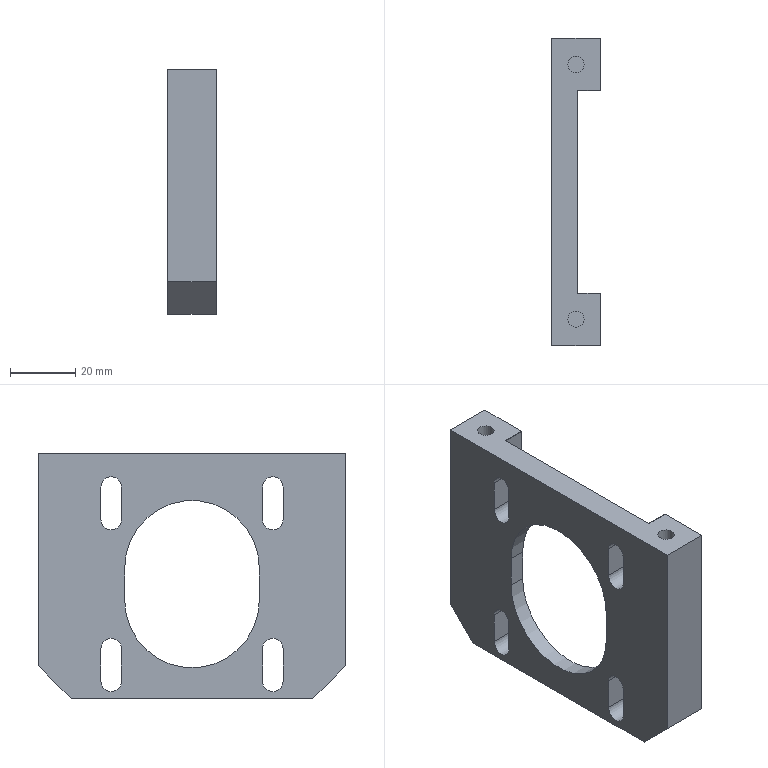Part | 1 solid | 45 faces | box 15 x 94 x 75 mm | volume 51821 mm3 | plane 31 | cylinder 14 | commonest cylinder face diameters 6.3 x8 5 x2 41.2 x2 50.6 x2
STEP:
#1=CARTESIAN_POINT('',(-74.806,502.943,-274.3));
#2=VERTEX_POINT('',#1);
#3=CARTESIAN_POINT('',(-77.306,502.943,-274.3));
#4=DIRECTION('',(0.,0.,1.));
#5=DIRECTION('',(1.,0.,0.));
#6=AXIS2_PLACEMENT_3D('',#3,#4,#5);
#7=CIRCLE('',#6,2.5);
#8=EDGE_CURVE('',#2,#2,#7,.T.);
#9=ORIENTED_EDGE('',*,*,#8,.T.);
#10=EDGE_LOOP('',(#9));
#11=FACE_BOUND('',#10,.T.);
#12=CARTESIAN_POINT('',(-74.806,502.943,-289.3));
#13=VERTEX_POINT('',#12);
#14=CARTESIAN_POINT('',(-77.306,502.943,-289.3));
#15=DIRECTION('',(0.,0.,-1.));
#16=DIRECTION('',(1.,0.,0.));
#17=AXIS2_PLACEMENT_3D('',#14,#15,#16);
#18=CIRCLE('',#17,2.5);
#19=EDGE_CURVE('',#13,#13,#18,.T.);
#20=ORIENTED_EDGE('',*,*,#19,.T.);
#21=EDGE_LOOP('',(#20));
#22=FACE_BOUND('',#21,.T.);
#23=CARTESIAN_POINT('',(-77.306,502.943,-274.3));
#24=DIRECTION('',(0.,0.,-1.));
#25=DIRECTION('',(1.,0.,0.));
#26=AXIS2_PLACEMENT_3D('',#23,#24,#25);
#27=CYLINDRICAL_SURFACE('',#26,2.5);
#28=ADVANCED_FACE('',(#11,#22),#27,.F.);
#29=ORIENTED_EDGE('',*,*,#19,.F.);
#30=EDGE_LOOP('',(#29));
#31=FACE_BOUND('',#30,.T.);
#32=CARTESIAN_POINT('',(-77.306,502.943,-289.3));
#33=DIRECTION('',(0.,0.,-1.));
#34=DIRECTION('',(-1.,0.,0.));
#35=AXIS2_PLACEMENT_3D('',#32,#33,#34);
#36=PLANE('',#35);
#37=ADVANCED_FACE('',(#31),#36,.F.);
#38=CARTESIAN_POINT('',(-74.806,424.943,-274.3));
#39=VERTEX_POINT('',#38);
#40=CARTESIAN_POINT('',(-77.306,424.943,-274.3));
#41=DIRECTION('',(0.,0.,1.));
#42=DIRECTION('',(1.,0.,0.));
#43=AXIS2_PLACEMENT_3D('',#40,#41,#42);
#44=CIRCLE('',#43,2.5);
#45=EDGE_CURVE('',#39,#39,#44,.T.);
#46=ORIENTED_EDGE('',*,*,#45,.T.);
#47=EDGE_LOOP('',(#46));
#48=FACE_BOUND('',#47,.T.);
#49=CARTESIAN_POINT('',(-79.806,424.943,-289.3));
#50=VERTEX_POINT('',#49);
#51=CARTESIAN_POINT('',(-77.306,424.943,-289.3));
#52=DIRECTION('',(0.,0.,-1.));
#53=DIRECTION('',(-1.,0.,0.));
#54=AXIS2_PLACEMENT_3D('',#51,#52,#53);
#55=CIRCLE('',#54,2.5);
#56=EDGE_CURVE('',#50,#50,#55,.T.);
#57=ORIENTED_EDGE('',*,*,#56,.T.);
#58=EDGE_LOOP('',(#57));
#59=FACE_BOUND('',#58,.T.);
#60=CARTESIAN_POINT('',(-77.306,424.943,-274.3));
#61=DIRECTION('',(0.,0.,-1.));
#62=DIRECTION('',(1.,0.,0.));
#63=AXIS2_PLACEMENT_3D('',#60,#61,#62);
#64=CYLINDRICAL_SURFACE('',#63,2.5);
#65=ADVANCED_FACE('',(#48,#59),#64,.F.);
#66=ORIENTED_EDGE('',*,*,#56,.F.);
#67=EDGE_LOOP('',(#66));
#68=FACE_BOUND('',#67,.T.);
#69=CARTESIAN_POINT('',(-77.306,502.943,-289.3));
#70=DIRECTION('',(0.,0.,-1.));
#71=DIRECTION('',(-1.,0.,0.));
#72=AXIS2_PLACEMENT_3D('',#69,#70,#71);
#73=PLANE('',#72);
#74=ADVANCED_FACE('',(#68),#73,.F.);
#75=CARTESIAN_POINT('',(-69.806,416.943,-339.3));
#76=VERTEX_POINT('',#75);
#77=CARTESIAN_POINT('',(-69.806,426.943,-349.3));
#78=VERTEX_POINT('',#77);
#79=CARTESIAN_POINT('',(-69.806,447.943,-370.3));
#80=DIRECTION('',(0.,0.7071,-0.7071));
#81=VECTOR('',#80,1000.);
#82=LINE('',#79,#81);
#83=EDGE_CURVE('',#76,#78,#82,.T.);
#84=ORIENTED_EDGE('',*,*,#83,.F.);
#85=CARTESIAN_POINT('',(-84.806,416.943,-339.3));
#86=VERTEX_POINT('',#85);
#87=CARTESIAN_POINT('',(-74.806,416.943,-339.3));
#88=DIRECTION('',(1.,0.,0.));
#89=VECTOR('',#88,1000.);
#90=LINE('',#87,#89);
#91=EDGE_CURVE('',#86,#76,#90,.T.);
#92=ORIENTED_EDGE('',*,*,#91,.F.);
#93=CARTESIAN_POINT('',(-84.806,426.943,-349.3));
#94=VERTEX_POINT('',#93);
#95=CARTESIAN_POINT('',(-84.806,447.943,-370.3));
#96=DIRECTION('',(0.,-0.7071,0.7071));
#97=VECTOR('',#96,1000.);
#98=LINE('',#95,#97);
#99=EDGE_CURVE('',#94,#86,#98,.T.);
#100=ORIENTED_EDGE('',*,*,#99,.F.);
#101=CARTESIAN_POINT('',(25.994,426.943,-349.3));
#102=DIRECTION('',(-1.,0.,0.));
#103=VECTOR('',#102,1000.);
#104=LINE('',#101,#103);
#105=EDGE_CURVE('',#78,#94,#104,.T.);
#106=ORIENTED_EDGE('',*,*,#105,.F.);
#107=EDGE_LOOP('',(#84,#92,#100,#106));
#108=FACE_BOUND('',#107,.T.);
#109=CARTESIAN_POINT('',(25.994,426.943,-349.3));
#110=DIRECTION('',(0.,0.7071,0.7071));
#111=DIRECTION('',(-1.,0.,0.));
#112=AXIS2_PLACEMENT_3D('',#109,#110,#111);
#113=PLANE('',#112);
#114=ADVANCED_FACE('',(#108),#113,.F.);
#115=CARTESIAN_POINT('',(-84.806,510.943,-339.3));
#116=VERTEX_POINT('',#115);
#117=CARTESIAN_POINT('',(-84.806,500.943,-349.3));
#118=VERTEX_POINT('',#117);
#119=CARTESIAN_POINT('',(-84.806,479.943,-370.3));
#120=DIRECTION('',(0.,-0.7071,-0.7071));
#121=VECTOR('',#120,1000.);
#122=LINE('',#119,#121);
#123=EDGE_CURVE('',#116,#118,#122,.T.);
#124=ORIENTED_EDGE('',*,*,#123,.F.);
#125=CARTESIAN_POINT('',(-69.806,510.943,-339.3));
#126=VERTEX_POINT('',#125);
#127=CARTESIAN_POINT('',(-74.806,510.943,-339.3));
#128=DIRECTION('',(-1.,0.,0.));
#129=VECTOR('',#128,1000.);
#130=LINE('',#127,#129);
#131=EDGE_CURVE('',#126,#116,#130,.T.);
#132=ORIENTED_EDGE('',*,*,#131,.F.);
#133=CARTESIAN_POINT('',(-69.806,500.943,-349.3));
#134=VERTEX_POINT('',#133);
#135=CARTESIAN_POINT('',(-69.806,479.943,-370.3));
#136=DIRECTION('',(0.,0.7071,0.7071));
#137=VECTOR('',#136,1000.);
#138=LINE('',#135,#137);
#139=EDGE_CURVE('',#134,#126,#138,.T.);
#140=ORIENTED_EDGE('',*,*,#139,.F.);
#141=CARTESIAN_POINT('',(25.994,500.943,-349.3));
#142=DIRECTION('',(1.,0.,0.));
#143=VECTOR('',#142,1000.);
#144=LINE('',#141,#143);
#145=EDGE_CURVE('',#118,#134,#144,.T.);
#146=ORIENTED_EDGE('',*,*,#145,.F.);
#147=EDGE_LOOP('',(#124,#132,#140,#146));
#148=FACE_BOUND('',#147,.T.);
#149=CARTESIAN_POINT('',(25.994,500.943,-349.3));
#150=DIRECTION('',(0.,-0.7071,0.7071));
#151=DIRECTION('',(1.,0.,0.));
#152=AXIS2_PLACEMENT_3D('',#149,#150,#151);
#153=PLANE('',#152);
#154=ADVANCED_FACE('',(#148),#153,.F.);
#155=CARTESIAN_POINT('',(-76.806,436.044,-344.049));
#156=VERTEX_POINT('',#155);
#157=CARTESIAN_POINT('',(-76.806,442.344,-344.049));
#158=VERTEX_POINT('',#157);
#159=CARTESIAN_POINT('',(-76.806,439.194,-344.049));
#160=DIRECTION('',(1.,0.,0.));
#161=DIRECTION('',(0.,1.,0.));
#162=AXIS2_PLACEMENT_3D('',#159,#160,#161);
#163=CIRCLE('',#162,3.15);
#164=EDGE_CURVE('',#156,#158,#163,.T.);
#165=ORIENTED_EDGE('',*,*,#164,.T.);
#166=CARTESIAN_POINT('',(-84.806,442.344,-344.049));
#167=VERTEX_POINT('',#166);
#168=CARTESIAN_POINT('',(-80.806,442.344,-344.049));
#169=DIRECTION('',(1.,0.,0.));
#170=VECTOR('',#169,1000.);
#171=LINE('',#168,#170);
#172=EDGE_CURVE('',#167,#158,#171,.T.);
#173=ORIENTED_EDGE('',*,*,#172,.F.);
#174=CARTESIAN_POINT('',(-84.806,436.044,-344.049));
#175=VERTEX_POINT('',#174);
#176=CARTESIAN_POINT('',(-84.806,439.194,-344.049));
#177=DIRECTION('',(-1.,0.,0.));
#178=DIRECTION('',(0.,-1.,0.));
#179=AXIS2_PLACEMENT_3D('',#176,#177,#178);
#180=CIRCLE('',#179,3.15);
#181=EDGE_CURVE('',#167,#175,#180,.T.);
#182=ORIENTED_EDGE('',*,*,#181,.T.);
#183=CARTESIAN_POINT('',(-80.806,436.044,-344.049));
#184=DIRECTION('',(-1.,0.,0.));
#185=VECTOR('',#184,1000.);
#186=LINE('',#183,#185);
#187=EDGE_CURVE('',#156,#175,#186,.T.);
#188=ORIENTED_EDGE('',*,*,#187,.F.);
#189=EDGE_LOOP('',(#165,#173,#182,#188));
#190=FACE_BOUND('',#189,.T.);
#191=CARTESIAN_POINT('',(-80.806,439.194,-344.049));
#192=DIRECTION('',(-1.,0.,0.));
#193=DIRECTION('',(0.,-1.,0.));
#194=AXIS2_PLACEMENT_3D('',#191,#192,#193);
#195=CYLINDRICAL_SURFACE('',#194,3.15);
#196=ADVANCED_FACE('',(#190),#195,.F.);
#197=CARTESIAN_POINT('',(-76.806,442.344,-334.049));
#198=VERTEX_POINT('',#197);
#199=CARTESIAN_POINT('',(-76.806,436.044,-334.049));
#200=VERTEX_POINT('',#199);
#201=CARTESIAN_POINT('',(-76.806,439.194,-334.049));
#202=DIRECTION('',(1.,0.,0.));
#203=DIRECTION('',(0.,1.,0.));
#204=AXIS2_PLACEMENT_3D('',#201,#202,#203);
#205=CIRCLE('',#204,3.15);
#206=EDGE_CURVE('',#198,#200,#205,.T.);
#207=ORIENTED_EDGE('',*,*,#206,.T.);
#208=CARTESIAN_POINT('',(-84.806,436.044,-334.049));
#209=VERTEX_POINT('',#208);
#210=CARTESIAN_POINT('',(-80.806,436.044,-334.049));
#211=DIRECTION('',(1.,0.,0.));
#212=VECTOR('',#211,1000.);
#213=LINE('',#210,#212);
#214=EDGE_CURVE('',#209,#200,#213,.T.);
#215=ORIENTED_EDGE('',*,*,#214,.F.);
#216=CARTESIAN_POINT('',(-84.806,442.344,-334.049));
#217=VERTEX_POINT('',#216);
#218=CARTESIAN_POINT('',(-84.806,439.194,-334.049));
#219=DIRECTION('',(-1.,0.,0.));
#220=DIRECTION('',(0.,-1.,0.));
#221=AXIS2_PLACEMENT_3D('',#218,#219,#220);
#222=CIRCLE('',#221,3.15);
#223=EDGE_CURVE('',#209,#217,#222,.T.);
#224=ORIENTED_EDGE('',*,*,#223,.T.);
#225=CARTESIAN_POINT('',(-80.806,442.344,-334.049));
#226=DIRECTION('',(-1.,0.,0.));
#227=VECTOR('',#226,1000.);
#228=LINE('',#225,#227);
#229=EDGE_CURVE('',#198,#217,#228,.T.);
#230=ORIENTED_EDGE('',*,*,#229,.F.);
#231=EDGE_LOOP('',(#207,#215,#224,#230));
#232=FACE_BOUND('',#231,.T.);
#233=CARTESIAN_POINT('',(-80.806,439.194,-334.049));
#234=DIRECTION('',(1.,0.,0.));
#235=DIRECTION('',(0.,1.,0.));
#236=AXIS2_PLACEMENT_3D('',#233,#234,#235);
#237=CYLINDRICAL_SURFACE('',#236,3.15);
#238=ADVANCED_FACE('',(#232),#237,.F.);
#239=CARTESIAN_POINT('',(-84.806,442.344,-339.049));
#240=DIRECTION('',(0.,0.,-1.));
#241=VECTOR('',#240,1000.);
#242=LINE('',#239,#241);
#243=EDGE_CURVE('',#217,#167,#242,.T.);
#244=ORIENTED_EDGE('',*,*,#243,.T.);
#245=ORIENTED_EDGE('',*,*,#172,.T.);
#246=CARTESIAN_POINT('',(-76.806,442.344,-354.3));
#247=DIRECTION('',(0.,0.,1.));
#248=VECTOR('',#247,1000.);
#249=LINE('',#246,#248);
#250=EDGE_CURVE('',#158,#198,#249,.T.);
#251=ORIENTED_EDGE('',*,*,#250,.T.);
#252=ORIENTED_EDGE('',*,*,#229,.T.);
#253=EDGE_LOOP('',(#244,#245,#251,#252));
#254=FACE_BOUND('',#253,.T.);
#255=CARTESIAN_POINT('',(-80.806,442.344,-339.049));
#256=DIRECTION('',(0.,1.,0.));
#257=DIRECTION('',(-1.,0.,0.));
#258=AXIS2_PLACEMENT_3D('',#255,#256,#257);
#259=PLANE('',#258);
#260=ADVANCED_FACE('',(#254),#259,.F.);
#261=CARTESIAN_POINT('',(-84.806,436.044,-339.049));
#262=DIRECTION('',(0.,0.,1.));
#263=VECTOR('',#262,1000.);
#264=LINE('',#261,#263);
#265=EDGE_CURVE('',#175,#209,#264,.T.);
#266=ORIENTED_EDGE('',*,*,#265,.T.);
#267=ORIENTED_EDGE('',*,*,#214,.T.);
#268=CARTESIAN_POINT('',(-76.806,436.044,-354.3));
#269=DIRECTION('',(0.,0.,-1.));
#270=VECTOR('',#269,1000.);
#271=LINE('',#268,#270);
#272=EDGE_CURVE('',#200,#156,#271,.T.);
#273=ORIENTED_EDGE('',*,*,#272,.T.);
#274=ORIENTED_EDGE('',*,*,#187,.T.);
#275=EDGE_LOOP('',(#266,#267,#273,#274));
#276=FACE_BOUND('',#275,.T.);
#277=CARTESIAN_POINT('',(-80.806,436.044,-339.049));
#278=DIRECTION('',(0.,-1.,0.));
#279=DIRECTION('',(1.,0.,0.));
#280=AXIS2_PLACEMENT_3D('',#277,#278,#279);
#281=PLANE('',#280);
#282=ADVANCED_FACE('',(#276),#281,.F.);
#283=CARTESIAN_POINT('',(-76.806,436.044,-294.551));
#284=VERTEX_POINT('',#283);
#285=CARTESIAN_POINT('',(-76.806,442.344,-294.551));
#286=VERTEX_POINT('',#285);
#287=CARTESIAN_POINT('',(-76.806,439.194,-294.551));
#288=DIRECTION('',(1.,0.,0.));
#289=DIRECTION('',(0.,1.,0.));
#290=AXIS2_PLACEMENT_3D('',#287,#288,#289);
#291=CIRCLE('',#290,3.15);
#292=EDGE_CURVE('',#284,#286,#291,.T.);
#293=ORIENTED_EDGE('',*,*,#292,.T.);
#294=CARTESIAN_POINT('',(-84.806,442.344,-294.551));
#295=VERTEX_POINT('',#294);
#296=CARTESIAN_POINT('',(-80.806,442.344,-294.551));
#297=DIRECTION('',(1.,0.,0.));
#298=VECTOR('',#297,1000.);
#299=LINE('',#296,#298);
#300=EDGE_CURVE('',#295,#286,#299,.T.);
#301=ORIENTED_EDGE('',*,*,#300,.F.);
#302=CARTESIAN_POINT('',(-84.806,436.044,-294.551));
#303=VERTEX_POINT('',#302);
#304=CARTESIAN_POINT('',(-84.806,439.194,-294.551));
#305=DIRECTION('',(-1.,0.,0.));
#306=DIRECTION('',(0.,-1.,0.));
#307=AXIS2_PLACEMENT_3D('',#304,#305,#306);
#308=CIRCLE('',#307,3.15);
#309=EDGE_CURVE('',#295,#303,#308,.T.);
#310=ORIENTED_EDGE('',*,*,#309,.T.);
#311=CARTESIAN_POINT('',(-80.806,436.044,-294.551));
#312=DIRECTION('',(-1.,0.,0.));
#313=VECTOR('',#312,1000.);
#314=LINE('',#311,#313);
#315=EDGE_CURVE('',#284,#303,#314,.T.);
#316=ORIENTED_EDGE('',*,*,#315,.F.);
#317=EDGE_LOOP('',(#293,#301,#310,#316));
#318=FACE_BOUND('',#317,.T.);
#319=CARTESIAN_POINT('',(-80.806,439.194,-294.551));
#320=DIRECTION('',(-1.,0.,0.));
#321=DIRECTION('',(0.,-1.,0.));
#322=AXIS2_PLACEMENT_3D('',#319,#320,#321);
#323=CYLINDRICAL_SURFACE('',#322,3.15);
#324=ADVANCED_FACE('',(#318),#323,.F.);
#325=CARTESIAN_POINT('',(-76.806,442.344,-284.551));
#326=VERTEX_POINT('',#325);
#327=CARTESIAN_POINT('',(-76.806,436.044,-284.551));
#328=VERTEX_POINT('',#327);
#329=CARTESIAN_POINT('',(-76.806,439.194,-284.551));
#330=DIRECTION('',(1.,0.,0.));
#331=DIRECTION('',(0.,1.,0.));
#332=AXIS2_PLACEMENT_3D('',#329,#330,#331);
#333=CIRCLE('',#332,3.15);
#334=EDGE_CURVE('',#326,#328,#333,.T.);
#335=ORIENTED_EDGE('',*,*,#334,.T.);
#336=CARTESIAN_POINT('',(-84.806,436.044,-284.551));
#337=VERTEX_POINT('',#336);
#338=CARTESIAN_POINT('',(-80.806,436.044,-284.551));
#339=DIRECTION('',(1.,0.,0.));
#340=VECTOR('',#339,1000.);
#341=LINE('',#338,#340);
#342=EDGE_CURVE('',#337,#328,#341,.T.);
#343=ORIENTED_EDGE('',*,*,#342,.F.);
#344=CARTESIAN_POINT('',(-84.806,442.344,-284.551));
#345=VERTEX_POINT('',#344);
#346=CARTESIAN_POINT('',(-84.806,439.194,-284.551));
#347=DIRECTION('',(-1.,0.,0.));
#348=DIRECTION('',(0.,-1.,0.));
#349=AXIS2_PLACEMENT_3D('',#346,#347,#348);
#350=CIRCLE('',#349,3.15);
#351=EDGE_CURVE('',#337,#345,#350,.T.);
#352=ORIENTED_EDGE('',*,*,#351,.T.);
#353=CARTESIAN_POINT('',(-80.806,442.344,-284.551));
#354=DIRECTION('',(-1.,0.,0.));
#355=VECTOR('',#354,1000.);
#356=LINE('',#353,#355);
#357=EDGE_CURVE('',#326,#345,#356,.T.);
#358=ORIENTED_EDGE('',*,*,#357,.F.);
#359=EDGE_LOOP('',(#335,#343,#352,#358));
#360=FACE_BOUND('',#359,.T.);
#361=CARTESIAN_POINT('',(-80.806,439.194,-284.551));
#362=DIRECTION('',(1.,0.,0.));
#363=DIRECTION('',(0.,1.,0.));
#364=AXIS2_PLACEMENT_3D('',#361,#362,#363);
#365=CYLINDRICAL_SURFACE('',#364,3.15);
#366=ADVANCED_FACE('',(#360),#365,.F.);
#367=CARTESIAN_POINT('',(-84.806,442.344,-339.049));
#368=DIRECTION('',(0.,0.,-1.));
#369=VECTOR('',#368,1000.);
#370=LINE('',#367,#369);
#371=EDGE_CURVE('',#345,#295,#370,.T.);
#372=ORIENTED_EDGE('',*,*,#371,.T.);
#373=ORIENTED_EDGE('',*,*,#300,.T.);
#374=CARTESIAN_POINT('',(-76.806,442.344,-339.049));
#375=DIRECTION('',(0.,0.,1.));
#376=VECTOR('',#375,1000.);
#377=LINE('',#374,#376);
#378=EDGE_CURVE('',#286,#326,#377,.T.);
#379=ORIENTED_EDGE('',*,*,#378,.T.);
#380=ORIENTED_EDGE('',*,*,#357,.T.);
#381=EDGE_LOOP('',(#372,#373,#379,#380));
#382=FACE_BOUND('',#381,.T.);
#383=CARTESIAN_POINT('',(-80.806,442.344,-339.049));
#384=DIRECTION('',(0.,1.,0.));
#385=DIRECTION('',(-1.,0.,0.));
#386=AXIS2_PLACEMENT_3D('',#383,#384,#385);
#387=PLANE('',#386);
#388=ADVANCED_FACE('',(#382),#387,.F.);
#389=CARTESIAN_POINT('',(-84.806,436.044,-339.049));
#390=DIRECTION('',(0.,0.,1.));
#391=VECTOR('',#390,1000.);
#392=LINE('',#389,#391);
#393=EDGE_CURVE('',#303,#337,#392,.T.);
#394=ORIENTED_EDGE('',*,*,#393,.T.);
#395=ORIENTED_EDGE('',*,*,#342,.T.);
#396=CARTESIAN_POINT('',(-76.806,436.044,-339.049));
#397=DIRECTION('',(0.,0.,-1.));
#398=VECTOR('',#397,1000.);
#399=LINE('',#396,#398);
#400=EDGE_CURVE('',#328,#284,#399,.T.);
#401=ORIENTED_EDGE('',*,*,#400,.T.);
#402=ORIENTED_EDGE('',*,*,#315,.T.);
#403=EDGE_LOOP('',(#394,#395,#401,#402));
#404=FACE_BOUND('',#403,.T.);
#405=CARTESIAN_POINT('',(-80.806,436.044,-339.049));
#406=DIRECTION('',(0.,-1.,0.));
#407=DIRECTION('',(1.,0.,0.));
#408=AXIS2_PLACEMENT_3D('',#405,#406,#407);
#409=PLANE('',#408);
#410=ADVANCED_FACE('',(#404),#409,.F.);
#411=CARTESIAN_POINT('',(-76.806,485.542,-344.049));
#412=VERTEX_POINT('',#411);
#413=CARTESIAN_POINT('',(-76.806,491.842,-344.049));
#414=VERTEX_POINT('',#413);
#415=CARTESIAN_POINT('',(-76.806,488.692,-344.049));
#416=DIRECTION('',(1.,0.,0.));
#417=DIRECTION('',(0.,1.,0.));
#418=AXIS2_PLACEMENT_3D('',#415,#416,#417);
#419=CIRCLE('',#418,3.15);
#420=EDGE_CURVE('',#412,#414,#419,.T.);
#421=ORIENTED_EDGE('',*,*,#420,.T.);
#422=CARTESIAN_POINT('',(-84.806,491.842,-344.049));
#423=VERTEX_POINT('',#422);
#424=CARTESIAN_POINT('',(-80.806,491.842,-344.049));
#425=DIRECTION('',(1.,0.,0.));
#426=VECTOR('',#425,1000.);
#427=LINE('',#424,#426);
#428=EDGE_CURVE('',#423,#414,#427,.T.);
#429=ORIENTED_EDGE('',*,*,#428,.F.);
#430=CARTESIAN_POINT('',(-84.806,485.542,-344.049));
#431=VERTEX_POINT('',#430);
#432=CARTESIAN_POINT('',(-84.806,488.692,-344.049));
#433=DIRECTION('',(-1.,0.,0.));
#434=DIRECTION('',(0.,-1.,0.));
#435=AXIS2_PLACEMENT_3D('',#432,#433,#434);
#436=CIRCLE('',#435,3.15);
#437=EDGE_CURVE('',#423,#431,#436,.T.);
#438=ORIENTED_EDGE('',*,*,#437,.T.);
#439=CARTESIAN_POINT('',(-80.806,485.542,-344.049));
#440=DIRECTION('',(-1.,0.,0.));
#441=VECTOR('',#440,1000.);
#442=LINE('',#439,#441);
#443=EDGE_CURVE('',#412,#431,#442,.T.);
#444=ORIENTED_EDGE('',*,*,#443,.F.);
#445=EDGE_LOOP('',(#421,#429,#438,#444));
#446=FACE_BOUND('',#445,.T.);
#447=CARTESIAN_POINT('',(-80.806,488.692,-344.049));
#448=DIRECTION('',(-1.,0.,0.));
#449=DIRECTION('',(0.,-1.,0.));
#450=AXIS2_PLACEMENT_3D('',#447,#448,#449);
#451=CYLINDRICAL_SURFACE('',#450,3.15);
#452=ADVANCED_FACE('',(#446),#451,.F.);
#453=CARTESIAN_POINT('',(-76.806,491.842,-334.049));
#454=VERTEX_POINT('',#453);
#455=CARTESIAN_POINT('',(-76.806,485.542,-334.049));
#456=VERTEX_POINT('',#455);
#457=CARTESIAN_POINT('',(-76.806,488.692,-334.049));
#458=DIRECTION('',(1.,0.,0.));
#459=DIRECTION('',(0.,1.,0.));
#460=AXIS2_PLACEMENT_3D('',#457,#458,#459);
#461=CIRCLE('',#460,3.15);
#462=EDGE_CURVE('',#454,#456,#461,.T.);
#463=ORIENTED_EDGE('',*,*,#462,.T.);
#464=CARTESIAN_POINT('',(-84.806,485.542,-334.049));
#465=VERTEX_POINT('',#464);
#466=CARTESIAN_POINT('',(-80.806,485.542,-334.049));
#467=DIRECTION('',(1.,0.,0.));
#468=VECTOR('',#467,1000.);
#469=LINE('',#466,#468);
#470=EDGE_CURVE('',#465,#456,#469,.T.);
#471=ORIENTED_EDGE('',*,*,#470,.F.);
#472=CARTESIAN_POINT('',(-84.806,491.842,-334.049));
#473=VERTEX_POINT('',#472);
#474=CARTESIAN_POINT('',(-84.806,488.692,-334.049));
#475=DIRECTION('',(-1.,0.,0.));
#476=DIRECTION('',(0.,-1.,0.));
#477=AXIS2_PLACEMENT_3D('',#474,#475,#476);
#478=CIRCLE('',#477,3.15);
#479=EDGE_CURVE('',#465,#473,#478,.T.);
#480=ORIENTED_EDGE('',*,*,#479,.T.);
#481=CARTESIAN_POINT('',(-80.806,491.842,-334.049));
#482=DIRECTION('',(-1.,0.,0.));
#483=VECTOR('',#482,1000.);
#484=LINE('',#481,#483);
#485=EDGE_CURVE('',#454,#473,#484,.T.);
#486=ORIENTED_EDGE('',*,*,#485,.F.);
#487=EDGE_LOOP('',(#463,#471,#480,#486));
#488=FACE_BOUND('',#487,.T.);
#489=CARTESIAN_POINT('',(-80.806,488.692,-334.049));
#490=DIRECTION('',(1.,0.,0.));
#491=DIRECTION('',(0.,1.,0.));
#492=AXIS2_PLACEMENT_3D('',#489,#490,#491);
#493=CYLINDRICAL_SURFACE('',#492,3.15);
#494=ADVANCED_FACE('',(#488),#493,.F.);
#495=CARTESIAN_POINT('',(-84.806,491.842,-339.049));
#496=DIRECTION('',(0.,0.,-1.));
#497=VECTOR('',#496,1000.);
#498=LINE('',#495,#497);
#499=EDGE_CURVE('',#473,#423,#498,.T.);
#500=ORIENTED_EDGE('',*,*,#499,.T.);
#501=ORIENTED_EDGE('',*,*,#428,.T.);
#502=CARTESIAN_POINT('',(-76.806,491.842,-354.3));
#503=DIRECTION('',(0.,0.,1.));
#504=VECTOR('',#503,1000.);
#505=LINE('',#502,#504);
#506=EDGE_CURVE('',#414,#454,#505,.T.);
#507=ORIENTED_EDGE('',*,*,#506,.T.);
#508=ORIENTED_EDGE('',*,*,#485,.T.);
#509=EDGE_LOOP('',(#500,#501,#507,#508));
#510=FACE_BOUND('',#509,.T.);
#511=CARTESIAN_POINT('',(-80.806,491.842,-339.049));
#512=DIRECTION('',(0.,1.,0.));
#513=DIRECTION('',(-1.,0.,0.));
#514=AXIS2_PLACEMENT_3D('',#511,#512,#513);
#515=PLANE('',#514);
#516=ADVANCED_FACE('',(#510),#515,.F.);
#517=CARTESIAN_POINT('',(-84.806,485.542,-339.049));
#518=DIRECTION('',(0.,0.,1.));
#519=VECTOR('',#518,1000.);
#520=LINE('',#517,#519);
#521=EDGE_CURVE('',#431,#465,#520,.T.);
#522=ORIENTED_EDGE('',*,*,#521,.T.);
#523=ORIENTED_EDGE('',*,*,#470,.T.);
#524=CARTESIAN_POINT('',(-76.806,485.542,-354.3));
#525=DIRECTION('',(0.,0.,-1.));
#526=VECTOR('',#525,1000.);
#527=LINE('',#524,#526);
#528=EDGE_CURVE('',#456,#412,#527,.T.);
#529=ORIENTED_EDGE('',*,*,#528,.T.);
#530=ORIENTED_EDGE('',*,*,#443,.T.);
#531=EDGE_LOOP('',(#522,#523,#529,#530));
#532=FACE_BOUND('',#531,.T.);
#533=CARTESIAN_POINT('',(-80.806,485.542,-339.049));
#534=DIRECTION('',(0.,-1.,0.));
#535=DIRECTION('',(1.,0.,0.));
#536=AXIS2_PLACEMENT_3D('',#533,#534,#535);
#537=PLANE('',#536);
#538=ADVANCED_FACE('',(#532),#537,.F.);
#539=CARTESIAN_POINT('',(-76.806,485.542,-294.551));
#540=VERTEX_POINT('',#539);
#541=CARTESIAN_POINT('',(-76.806,491.842,-294.551));
#542=VERTEX_POINT('',#541);
#543=CARTESIAN_POINT('',(-76.806,488.692,-294.551));
#544=DIRECTION('',(1.,0.,0.));
#545=DIRECTION('',(0.,1.,0.));
#546=AXIS2_PLACEMENT_3D('',#543,#544,#545);
#547=CIRCLE('',#546,3.15);
#548=EDGE_CURVE('',#540,#542,#547,.T.);
#549=ORIENTED_EDGE('',*,*,#548,.T.);
#550=CARTESIAN_POINT('',(-84.806,491.842,-294.551));
#551=VERTEX_POINT('',#550);
#552=CARTESIAN_POINT('',(-80.806,491.842,-294.551));
#553=DIRECTION('',(1.,0.,0.));
#554=VECTOR('',#553,1000.);
#555=LINE('',#552,#554);
#556=EDGE_CURVE('',#551,#542,#555,.T.);
#557=ORIENTED_EDGE('',*,*,#556,.F.);
#558=CARTESIAN_POINT('',(-84.806,485.542,-294.551));
#559=VERTEX_POINT('',#558);
#560=CARTESIAN_POINT('',(-84.806,488.692,-294.551));
#561=DIRECTION('',(-1.,0.,0.));
#562=DIRECTION('',(0.,-1.,0.));
#563=AXIS2_PLACEMENT_3D('',#560,#561,#562);
#564=CIRCLE('',#563,3.15);
#565=EDGE_CURVE('',#551,#559,#564,.T.);
#566=ORIENTED_EDGE('',*,*,#565,.T.);
#567=CARTESIAN_POINT('',(-80.806,485.542,-294.551));
#568=DIRECTION('',(-1.,0.,0.));
#569=VECTOR('',#568,1000.);
#570=LINE('',#567,#569);
#571=EDGE_CURVE('',#540,#559,#570,.T.);
#572=ORIENTED_EDGE('',*,*,#571,.F.);
#573=EDGE_LOOP('',(#549,#557,#566,#572));
#574=FACE_BOUND('',#573,.T.);
#575=CARTESIAN_POINT('',(-80.806,488.692,-294.551));
#576=DIRECTION('',(-1.,0.,0.));
#577=DIRECTION('',(0.,-1.,0.));
#578=AXIS2_PLACEMENT_3D('',#575,#576,#577);
#579=CYLINDRICAL_SURFACE('',#578,3.15);
#580=ADVANCED_FACE('',(#574),#579,.F.);
#581=CARTESIAN_POINT('',(-76.806,491.842,-284.551));
#582=VERTEX_POINT('',#581);
#583=CARTESIAN_POINT('',(-76.806,485.542,-284.551));
#584=VERTEX_POINT('',#583);
#585=CARTESIAN_POINT('',(-76.806,488.692,-284.551));
#586=DIRECTION('',(1.,0.,0.));
#587=DIRECTION('',(0.,1.,0.));
#588=AXIS2_PLACEMENT_3D('',#585,#586,#587);
#589=CIRCLE('',#588,3.15);
#590=EDGE_CURVE('',#582,#584,#589,.T.);
#591=ORIENTED_EDGE('',*,*,#590,.T.);
#592=CARTESIAN_POINT('',(-84.806,485.542,-284.551));
#593=VERTEX_POINT('',#592);
#594=CARTESIAN_POINT('',(-80.806,485.542,-284.551));
#595=DIRECTION('',(1.,0.,0.));
#596=VECTOR('',#595,1000.);
#597=LINE('',#594,#596);
#598=EDGE_CURVE('',#593,#584,#597,.T.);
#599=ORIENTED_EDGE('',*,*,#598,.F.);
#600=CARTESIAN_POINT('',(-84.806,491.842,-284.551));
#601=VERTEX_POINT('',#600);
#602=CARTESIAN_POINT('',(-84.806,488.692,-284.551));
#603=DIRECTION('',(-1.,0.,0.));
#604=DIRECTION('',(0.,-1.,0.));
#605=AXIS2_PLACEMENT_3D('',#602,#603,#604);
#606=CIRCLE('',#605,3.15);
#607=EDGE_CURVE('',#593,#601,#606,.T.);
#608=ORIENTED_EDGE('',*,*,#607,.T.);
#609=CARTESIAN_POINT('',(-80.806,491.842,-284.551));
#610=DIRECTION('',(-1.,0.,0.));
#611=VECTOR('',#610,1000.);
#612=LINE('',#609,#611);
#613=EDGE_CURVE('',#582,#601,#612,.T.);
#614=ORIENTED_EDGE('',*,*,#613,.F.);
#615=EDGE_LOOP('',(#591,#599,#608,#614));
#616=FACE_BOUND('',#615,.T.);
#617=CARTESIAN_POINT('',(-80.806,488.692,-284.551));
#618=DIRECTION('',(1.,0.,0.));
#619=DIRECTION('',(0.,1.,0.));
#620=AXIS2_PLACEMENT_3D('',#617,#618,#619);
#621=CYLINDRICAL_SURFACE('',#620,3.15);
#622=ADVANCED_FACE('',(#616),#621,.F.);
#623=CARTESIAN_POINT('',(-84.806,491.842,-339.049));
#624=DIRECTION('',(0.,0.,-1.));
#625=VECTOR('',#624,1000.);
#626=LINE('',#623,#625);
#627=EDGE_CURVE('',#601,#551,#626,.T.);
#628=ORIENTED_EDGE('',*,*,#627,.T.);
#629=ORIENTED_EDGE('',*,*,#556,.T.);
#630=CARTESIAN_POINT('',(-76.806,491.842,-339.049));
#631=DIRECTION('',(0.,0.,1.));
#632=VECTOR('',#631,1000.);
#633=LINE('',#630,#632);
#634=EDGE_CURVE('',#542,#582,#633,.T.);
#635=ORIENTED_EDGE('',*,*,#634,.T.);
#636=ORIENTED_EDGE('',*,*,#613,.T.);
#637=EDGE_LOOP('',(#628,#629,#635,#636));
#638=FACE_BOUND('',#637,.T.);
#639=CARTESIAN_POINT('',(-80.806,491.842,-339.049));
#640=DIRECTION('',(0.,1.,0.));
#641=DIRECTION('',(-1.,0.,0.));
#642=AXIS2_PLACEMENT_3D('',#639,#640,#641);
#643=PLANE('',#642);
#644=ADVANCED_FACE('',(#638),#643,.F.);
#645=CARTESIAN_POINT('',(-84.806,485.542,-339.049));
#646=DIRECTION('',(0.,0.,1.));
#647=VECTOR('',#646,1000.);
#648=LINE('',#645,#647);
#649=EDGE_CURVE('',#559,#593,#648,.T.);
#650=ORIENTED_EDGE('',*,*,#649,.T.);
#651=ORIENTED_EDGE('',*,*,#598,.T.);
#652=CARTESIAN_POINT('',(-76.806,485.542,-339.049));
#653=DIRECTION('',(0.,0.,-1.));
#654=VECTOR('',#653,1000.);
#655=LINE('',#652,#654);
#656=EDGE_CURVE('',#584,#540,#655,.T.);
#657=ORIENTED_EDGE('',*,*,#656,.T.);
#658=ORIENTED_EDGE('',*,*,#571,.T.);
#659=EDGE_LOOP('',(#650,#651,#657,#658));
#660=FACE_BOUND('',#659,.T.);
#661=CARTESIAN_POINT('',(-80.806,485.542,-339.049));
#662=DIRECTION('',(0.,-1.,0.));
#663=DIRECTION('',(1.,0.,0.));
#664=AXIS2_PLACEMENT_3D('',#661,#662,#663);
#665=PLANE('',#664);
#666=ADVANCED_FACE('',(#660),#665,.F.);
#667=CARTESIAN_POINT('',(-84.806,443.343,-309.3));
#668=VERTEX_POINT('',#667);
#669=CARTESIAN_POINT('',(-79.806,443.343,-309.3));
#670=VERTEX_POINT('',#669);
#671=CARTESIAN_POINT('',(-82.306,443.343,-309.3));
#672=DIRECTION('',(1.,0.,0.));
#673=VECTOR('',#672,1000.);
#674=LINE('',#671,#673);
#675=EDGE_CURVE('',#668,#670,#674,.T.);
#676=ORIENTED_EDGE('',*,*,#675,.F.);
#677=CARTESIAN_POINT('',(-84.806,484.543,-309.3));
#678=VERTEX_POINT('',#677);
#679=CARTESIAN_POINT('',(-84.806,463.943,-309.3));
#680=DIRECTION('',(-1.,0.,0.));
#681=DIRECTION('',(0.,-1.,0.));
#682=AXIS2_PLACEMENT_3D('',#679,#680,#681);
#683=CIRCLE('',#682,20.6);
#684=EDGE_CURVE('',#668,#678,#683,.T.);
#685=ORIENTED_EDGE('',*,*,#684,.T.);
#686=CARTESIAN_POINT('',(-79.806,484.543,-309.3));
#687=VERTEX_POINT('',#686);
#688=CARTESIAN_POINT('',(-82.306,484.543,-309.3));
#689=DIRECTION('',(-1.,0.,0.));
#690=VECTOR('',#689,1000.);
#691=LINE('',#688,#690);
#692=EDGE_CURVE('',#687,#678,#691,.T.);
#693=ORIENTED_EDGE('',*,*,#692,.F.);
#694=CARTESIAN_POINT('',(-79.806,463.943,-309.3));
#695=DIRECTION('',(1.,0.,0.));
#696=DIRECTION('',(0.,1.,0.));
#697=AXIS2_PLACEMENT_3D('',#694,#695,#696);
#698=CIRCLE('',#697,20.6);
#699=EDGE_CURVE('',#687,#670,#698,.T.);
#700=ORIENTED_EDGE('',*,*,#699,.T.);
#701=EDGE_LOOP('',(#676,#685,#693,#700));
#702=FACE_BOUND('',#701,.T.);
#703=CARTESIAN_POINT('',(-82.306,463.943,-309.3));
#704=DIRECTION('',(1.,0.,0.));
#705=DIRECTION('',(0.,1.,0.));
#706=AXIS2_PLACEMENT_3D('',#703,#704,#705);
#707=CYLINDRICAL_SURFACE('',#706,20.6);
#708=ADVANCED_FACE('',(#702),#707,.F.);
#709=CARTESIAN_POINT('',(-84.806,484.543,-319.3));
#710=VERTEX_POINT('',#709);
#711=CARTESIAN_POINT('',(-79.806,484.543,-319.3));
#712=VERTEX_POINT('',#711);
#713=CARTESIAN_POINT('',(-82.306,484.543,-319.3));
#714=DIRECTION('',(1.,0.,0.));
#715=VECTOR('',#714,1000.);
#716=LINE('',#713,#715);
#717=EDGE_CURVE('',#710,#712,#716,.T.);
#718=ORIENTED_EDGE('',*,*,#717,.F.);
#719=CARTESIAN_POINT('',(-84.806,443.343,-319.3));
#720=VERTEX_POINT('',#719);
#721=CARTESIAN_POINT('',(-84.806,463.943,-319.3));
#722=DIRECTION('',(-1.,0.,0.));
#723=DIRECTION('',(0.,-1.,0.));
#724=AXIS2_PLACEMENT_3D('',#721,#722,#723);
#725=CIRCLE('',#724,20.6);
#726=EDGE_CURVE('',#710,#720,#725,.T.);
#727=ORIENTED_EDGE('',*,*,#726,.T.);
#728=CARTESIAN_POINT('',(-79.806,443.343,-319.3));
#729=VERTEX_POINT('',#728);
#730=CARTESIAN_POINT('',(-82.306,443.343,-319.3));
#731=DIRECTION('',(-1.,0.,0.));
#732=VECTOR('',#731,1000.);
#733=LINE('',#730,#732);
#734=EDGE_CURVE('',#729,#720,#733,.T.);
#735=ORIENTED_EDGE('',*,*,#734,.F.);
#736=CARTESIAN_POINT('',(-79.806,463.943,-319.3));
#737=DIRECTION('',(1.,0.,0.));
#738=DIRECTION('',(0.,1.,0.));
#739=AXIS2_PLACEMENT_3D('',#736,#737,#738);
#740=CIRCLE('',#739,20.6);
#741=EDGE_CURVE('',#729,#712,#740,.T.);
#742=ORIENTED_EDGE('',*,*,#741,.T.);
#743=EDGE_LOOP('',(#718,#727,#735,#742));
#744=FACE_BOUND('',#743,.T.);
#745=CARTESIAN_POINT('',(-82.306,463.943,-319.3));
#746=DIRECTION('',(1.,0.,0.));
#747=DIRECTION('',(0.,1.,0.));
#748=AXIS2_PLACEMENT_3D('',#745,#746,#747);
#749=CYLINDRICAL_SURFACE('',#748,20.6);
#750=ADVANCED_FACE('',(#744),#749,.F.);
#751=CARTESIAN_POINT('',(-84.806,484.543,-314.3));
#752=DIRECTION('',(0.,0.,-1.));
#753=VECTOR('',#752,1000.);
#754=LINE('',#751,#753);
#755=EDGE_CURVE('',#678,#710,#754,.T.);
#756=ORIENTED_EDGE('',*,*,#755,.T.);
#757=ORIENTED_EDGE('',*,*,#717,.T.);
#758=CARTESIAN_POINT('',(-79.806,484.543,-314.3));
#759=DIRECTION('',(0.,0.,1.));
#760=VECTOR('',#759,1000.);
#761=LINE('',#758,#760);
#762=EDGE_CURVE('',#712,#687,#761,.T.);
#763=ORIENTED_EDGE('',*,*,#762,.T.);
#764=ORIENTED_EDGE('',*,*,#692,.T.);
#765=EDGE_LOOP('',(#756,#757,#763,#764));
#766=FACE_BOUND('',#765,.T.);
#767=CARTESIAN_POINT('',(-82.306,484.543,-314.3));
#768=DIRECTION('',(0.,1.,0.));
#769=DIRECTION('',(-1.,0.,0.));
#770=AXIS2_PLACEMENT_3D('',#767,#768,#769);
#771=PLANE('',#770);
#772=ADVANCED_FACE('',(#766),#771,.F.);
#773=CARTESIAN_POINT('',(-84.806,443.343,-314.3));
#774=DIRECTION('',(0.,0.,1.));
#775=VECTOR('',#774,1000.);
#776=LINE('',#773,#775);
#777=EDGE_CURVE('',#720,#668,#776,.T.);
#778=ORIENTED_EDGE('',*,*,#777,.T.);
#779=ORIENTED_EDGE('',*,*,#675,.T.);
#780=CARTESIAN_POINT('',(-79.806,443.343,-314.3));
#781=DIRECTION('',(0.,0.,-1.));
#782=VECTOR('',#781,1000.);
#783=LINE('',#780,#782);
#784=EDGE_CURVE('',#670,#729,#783,.T.);
#785=ORIENTED_EDGE('',*,*,#784,.T.);
#786=ORIENTED_EDGE('',*,*,#734,.T.);
#787=EDGE_LOOP('',(#778,#779,#785,#786));
#788=FACE_BOUND('',#787,.T.);
#789=CARTESIAN_POINT('',(-82.306,443.343,-314.3));
#790=DIRECTION('',(0.,-1.,0.));
#791=DIRECTION('',(1.,0.,0.));
#792=AXIS2_PLACEMENT_3D('',#789,#790,#791);
#793=PLANE('',#792);
#794=ADVANCED_FACE('',(#788),#793,.F.);
#795=CARTESIAN_POINT('',(-76.806,438.643,-319.3));
#796=VERTEX_POINT('',#795);
#797=CARTESIAN_POINT('',(-79.806,438.643,-319.3));
#798=VERTEX_POINT('',#797);
#799=CARTESIAN_POINT('',(-78.306,438.643,-319.3));
#800=DIRECTION('',(-1.,0.,0.));
#801=VECTOR('',#800,1000.);
#802=LINE('',#799,#801);
#803=EDGE_CURVE('',#796,#798,#802,.T.);
#804=ORIENTED_EDGE('',*,*,#803,.F.);
#805=CARTESIAN_POINT('',(-76.806,489.243,-319.3));
#806=VERTEX_POINT('',#805);
#807=CARTESIAN_POINT('',(-76.806,463.943,-319.3));
#808=DIRECTION('',(1.,0.,0.));
#809=DIRECTION('',(0.,1.,0.));
#810=AXIS2_PLACEMENT_3D('',#807,#808,#809);
#811=CIRCLE('',#810,25.3);
#812=EDGE_CURVE('',#796,#806,#811,.T.);
#813=ORIENTED_EDGE('',*,*,#812,.T.);
#814=CARTESIAN_POINT('',(-79.806,489.243,-319.3));
#815=VERTEX_POINT('',#814);
#816=CARTESIAN_POINT('',(-78.306,489.243,-319.3));
#817=DIRECTION('',(1.,0.,0.));
#818=VECTOR('',#817,1000.);
#819=LINE('',#816,#818);
#820=EDGE_CURVE('',#815,#806,#819,.T.);
#821=ORIENTED_EDGE('',*,*,#820,.F.);
#822=CARTESIAN_POINT('',(-79.806,463.943,-319.3));
#823=DIRECTION('',(-1.,0.,0.));
#824=DIRECTION('',(0.,-1.,0.));
#825=AXIS2_PLACEMENT_3D('',#822,#823,#824);
#826=CIRCLE('',#825,25.3);
#827=EDGE_CURVE('',#815,#798,#826,.T.);
#828=ORIENTED_EDGE('',*,*,#827,.T.);
#829=EDGE_LOOP('',(#804,#813,#821,#828));
#830=FACE_BOUND('',#829,.T.);
#831=CARTESIAN_POINT('',(-78.306,463.943,-319.3));
#832=DIRECTION('',(-1.,0.,0.));
#833=DIRECTION('',(0.,-1.,0.));
#834=AXIS2_PLACEMENT_3D('',#831,#832,#833);
#835=CYLINDRICAL_SURFACE('',#834,25.3);
#836=ADVANCED_FACE('',(#830),#835,.F.);
#837=CARTESIAN_POINT('',(-79.806,438.643,-309.3));
#838=VERTEX_POINT('',#837);
#839=CARTESIAN_POINT('',(-76.806,438.643,-309.3));
#840=VERTEX_POINT('',#839);
#841=CARTESIAN_POINT('',(-78.306,438.643,-309.3));
#842=DIRECTION('',(1.,0.,0.));
#843=VECTOR('',#842,1000.);
#844=LINE('',#841,#843);
#845=EDGE_CURVE('',#838,#840,#844,.T.);
#846=ORIENTED_EDGE('',*,*,#845,.F.);
#847=CARTESIAN_POINT('',(-79.806,489.243,-309.3));
#848=VERTEX_POINT('',#847);
#849=CARTESIAN_POINT('',(-79.806,463.943,-309.3));
#850=DIRECTION('',(-1.,0.,0.));
#851=DIRECTION('',(0.,-1.,0.));
#852=AXIS2_PLACEMENT_3D('',#849,#850,#851);
#853=CIRCLE('',#852,25.3);
#854=EDGE_CURVE('',#838,#848,#853,.T.);
#855=ORIENTED_EDGE('',*,*,#854,.T.);
#856=CARTESIAN_POINT('',(-76.806,489.243,-309.3));
#857=VERTEX_POINT('',#856);
#858=CARTESIAN_POINT('',(-78.306,489.243,-309.3));
#859=DIRECTION('',(-1.,0.,0.));
#860=VECTOR('',#859,1000.);
#861=LINE('',#858,#860);
#862=EDGE_CURVE('',#857,#848,#861,.T.);
#863=ORIENTED_EDGE('',*,*,#862,.F.);
#864=CARTESIAN_POINT('',(-76.806,463.943,-309.3));
#865=DIRECTION('',(1.,0.,0.));
#866=DIRECTION('',(0.,1.,0.));
#867=AXIS2_PLACEMENT_3D('',#864,#865,#866);
#868=CIRCLE('',#867,25.3);
#869=EDGE_CURVE('',#857,#840,#868,.T.);
#870=ORIENTED_EDGE('',*,*,#869,.T.);
#871=EDGE_LOOP('',(#846,#855,#863,#870));
#872=FACE_BOUND('',#871,.T.);
#873=CARTESIAN_POINT('',(-78.306,463.943,-309.3));
#874=DIRECTION('',(1.,0.,0.));
#875=DIRECTION('',(0.,1.,0.));
#876=AXIS2_PLACEMENT_3D('',#873,#874,#875);
#877=CYLINDRICAL_SURFACE('',#876,25.3);
#878=ADVANCED_FACE('',(#872),#877,.F.);
#879=CARTESIAN_POINT('',(-79.806,489.243,-314.3));
#880=DIRECTION('',(0.,0.,-1.));
#881=VECTOR('',#880,1000.);
#882=LINE('',#879,#881);
#883=EDGE_CURVE('',#848,#815,#882,.T.);
#884=ORIENTED_EDGE('',*,*,#883,.T.);
#885=ORIENTED_EDGE('',*,*,#820,.T.);
#886=CARTESIAN_POINT('',(-76.806,489.243,-314.3));
#887=DIRECTION('',(0.,0.,1.));
#888=VECTOR('',#887,1000.);
#889=LINE('',#886,#888);
#890=EDGE_CURVE('',#806,#857,#889,.T.);
#891=ORIENTED_EDGE('',*,*,#890,.T.);
#892=ORIENTED_EDGE('',*,*,#862,.T.);
#893=EDGE_LOOP('',(#884,#885,#891,#892));
#894=FACE_BOUND('',#893,.T.);
#895=CARTESIAN_POINT('',(-78.306,489.243,-314.3));
#896=DIRECTION('',(0.,1.,0.));
#897=DIRECTION('',(-1.,0.,0.));
#898=AXIS2_PLACEMENT_3D('',#895,#896,#897);
#899=PLANE('',#898);
#900=ADVANCED_FACE('',(#894),#899,.F.);
#901=CARTESIAN_POINT('',(-79.806,438.643,-314.3));
#902=DIRECTION('',(0.,0.,1.));
#903=VECTOR('',#902,1000.);
#904=LINE('',#901,#903);
#905=EDGE_CURVE('',#798,#838,#904,.T.);
#906=ORIENTED_EDGE('',*,*,#905,.T.);
#907=ORIENTED_EDGE('',*,*,#845,.T.);
#908=CARTESIAN_POINT('',(-76.806,438.643,-314.3));
#909=DIRECTION('',(0.,0.,-1.));
#910=VECTOR('',#909,1000.);
#911=LINE('',#908,#910);
#912=EDGE_CURVE('',#840,#796,#911,.T.);
#913=ORIENTED_EDGE('',*,*,#912,.T.);
#914=ORIENTED_EDGE('',*,*,#803,.T.);
#915=EDGE_LOOP('',(#906,#907,#913,#914));
#916=FACE_BOUND('',#915,.T.);
#917=CARTESIAN_POINT('',(-78.306,438.643,-314.3));
#918=DIRECTION('',(0.,-1.,0.));
#919=DIRECTION('',(1.,0.,0.));
#920=AXIS2_PLACEMENT_3D('',#917,#918,#919);
#921=PLANE('',#920);
#922=ADVANCED_FACE('',(#916),#921,.F.);
#923=CARTESIAN_POINT('',(-84.806,510.943,-274.3));
#924=VERTEX_POINT('',#923);
#925=CARTESIAN_POINT('',(-84.806,510.943,-354.3));
#926=DIRECTION('',(0.,0.,1.));
#927=VECTOR('',#926,1000.);
#928=LINE('',#925,#927);
#929=EDGE_CURVE('',#116,#924,#928,.T.);
#930=ORIENTED_EDGE('',*,*,#929,.F.);
#931=ORIENTED_EDGE('',*,*,#123,.T.);
#932=CARTESIAN_POINT('',(-84.806,463.943,-349.3));
#933=DIRECTION('',(0.,-1.,0.));
#934=VECTOR('',#933,1000.);
#935=LINE('',#932,#934);
#936=EDGE_CURVE('',#118,#94,#935,.T.);
#937=ORIENTED_EDGE('',*,*,#936,.T.);
#938=ORIENTED_EDGE('',*,*,#99,.T.);
#939=CARTESIAN_POINT('',(-84.806,416.943,-274.3));
#940=VERTEX_POINT('',#939);
#941=CARTESIAN_POINT('',(-84.806,416.943,-354.3));
#942=DIRECTION('',(0.,0.,1.));
#943=VECTOR('',#942,1000.);
#944=LINE('',#941,#943);
#945=EDGE_CURVE('',#86,#940,#944,.T.);
#946=ORIENTED_EDGE('',*,*,#945,.T.);
#947=CARTESIAN_POINT('',(-84.806,463.943,-274.3));
#948=DIRECTION('',(0.,1.,0.));
#949=VECTOR('',#948,1000.);
#950=LINE('',#947,#949);
#951=EDGE_CURVE('',#940,#924,#950,.T.);
#952=ORIENTED_EDGE('',*,*,#951,.T.);
#953=EDGE_LOOP('',(#930,#931,#937,#938,#946,#952));
#954=FACE_BOUND('',#953,.T.);
#955=ORIENTED_EDGE('',*,*,#726,.F.);
#956=ORIENTED_EDGE('',*,*,#755,.F.);
#957=ORIENTED_EDGE('',*,*,#684,.F.);
#958=ORIENTED_EDGE('',*,*,#777,.F.);
#959=EDGE_LOOP('',(#955,#956,#957,#958));
#960=FACE_BOUND('',#959,.T.);
#961=ORIENTED_EDGE('',*,*,#607,.F.);
#962=ORIENTED_EDGE('',*,*,#649,.F.);
#963=ORIENTED_EDGE('',*,*,#565,.F.);
#964=ORIENTED_EDGE('',*,*,#627,.F.);
#965=EDGE_LOOP('',(#961,#962,#963,#964));
#966=FACE_BOUND('',#965,.T.);
#967=ORIENTED_EDGE('',*,*,#479,.F.);
#968=ORIENTED_EDGE('',*,*,#521,.F.);
#969=ORIENTED_EDGE('',*,*,#437,.F.);
#970=ORIENTED_EDGE('',*,*,#499,.F.);
#971=EDGE_LOOP('',(#967,#968,#969,#970));
#972=FACE_BOUND('',#971,.T.);
#973=ORIENTED_EDGE('',*,*,#351,.F.);
#974=ORIENTED_EDGE('',*,*,#393,.F.);
#975=ORIENTED_EDGE('',*,*,#309,.F.);
#976=ORIENTED_EDGE('',*,*,#371,.F.);
#977=EDGE_LOOP('',(#973,#974,#975,#976));
#978=FACE_BOUND('',#977,.T.);
#979=ORIENTED_EDGE('',*,*,#223,.F.);
#980=ORIENTED_EDGE('',*,*,#265,.F.);
#981=ORIENTED_EDGE('',*,*,#181,.F.);
#982=ORIENTED_EDGE('',*,*,#243,.F.);
#983=EDGE_LOOP('',(#979,#980,#981,#982));
#984=FACE_BOUND('',#983,.T.);
#985=CARTESIAN_POINT('',(-84.806,463.943,-354.3));
#986=DIRECTION('',(-1.,0.,0.));
#987=DIRECTION('',(0.,0.,1.));
#988=AXIS2_PLACEMENT_3D('',#985,#986,#987);
#989=PLANE('',#988);
#990=ADVANCED_FACE('',(#954,#960,#966,#972,#978,#984),#989,.T.);
#991=CARTESIAN_POINT('',(-69.806,432.943,-349.2));
#992=VERTEX_POINT('',#991);
#993=CARTESIAN_POINT('',(-69.806,432.943,-274.4));
#994=VERTEX_POINT('',#993);
#995=CARTESIAN_POINT('',(-69.806,432.943,-314.3));
#996=DIRECTION('',(0.,0.,1.));
#997=VECTOR('',#996,1000.);
#998=LINE('',#995,#997);
#999=EDGE_CURVE('',#992,#994,#998,.T.);
#1000=ORIENTED_EDGE('',*,*,#999,.F.);
#1001=CARTESIAN_POINT('',(-76.806,432.943,-349.2));
#1002=VERTEX_POINT('',#1001);
#1003=CARTESIAN_POINT('',(-76.806,432.943,-349.2));
#1004=DIRECTION('',(-1.,0.,0.));
#1005=VECTOR('',#1004,1000.);
#1006=LINE('',#1003,#1005);
#1007=EDGE_CURVE('',#992,#1002,#1006,.T.);
#1008=ORIENTED_EDGE('',*,*,#1007,.T.);
#1009=CARTESIAN_POINT('',(-76.806,432.943,-274.4));
#1010=VERTEX_POINT('',#1009);
#1011=CARTESIAN_POINT('',(-76.806,432.943,-354.3));
#1012=DIRECTION('',(0.,0.,-1.));
#1013=VECTOR('',#1012,1000.);
#1014=LINE('',#1011,#1013);
#1015=EDGE_CURVE('',#1010,#1002,#1014,.T.);
#1016=ORIENTED_EDGE('',*,*,#1015,.F.);
#1017=CARTESIAN_POINT('',(-43.106,432.943,-274.4));
#1018=DIRECTION('',(1.,0.,0.));
#1019=VECTOR('',#1018,1000.);
#1020=LINE('',#1017,#1019);
#1021=EDGE_CURVE('',#1010,#994,#1020,.T.);
#1022=ORIENTED_EDGE('',*,*,#1021,.T.);
#1023=EDGE_LOOP('',(#1000,#1008,#1016,#1022));
#1024=FACE_BOUND('',#1023,.T.);
#1025=CARTESIAN_POINT('',(-43.106,432.943,-314.3));
#1026=DIRECTION('',(0.,-1.,0.));
#1027=DIRECTION('',(1.,0.,0.));
#1028=AXIS2_PLACEMENT_3D('',#1025,#1026,#1027);
#1029=PLANE('',#1028);
#1030=ADVANCED_FACE('',(#1024),#1029,.F.);
#1031=CARTESIAN_POINT('',(-69.806,432.843,-349.3));
#1032=VERTEX_POINT('',#1031);
#1033=CARTESIAN_POINT('',(-69.806,463.943,-349.3));
#1034=DIRECTION('',(0.,1.,0.));
#1035=VECTOR('',#1034,1000.);
#1036=LINE('',#1033,#1035);
#1037=EDGE_CURVE('',#78,#1032,#1036,.T.);
#1038=ORIENTED_EDGE('',*,*,#1037,.T.);
#1039=CARTESIAN_POINT('',(-69.806,445.893,-336.25));
#1040=DIRECTION('',(0.,0.7071,0.7071));
#1041=VECTOR('',#1040,1000.);
#1042=LINE('',#1039,#1041);
#1043=EDGE_CURVE('',#1032,#992,#1042,.T.);
#1044=ORIENTED_EDGE('',*,*,#1043,.T.);
#1045=ORIENTED_EDGE('',*,*,#999,.T.);
#1046=CARTESIAN_POINT('',(-69.806,432.843,-274.3));
#1047=VERTEX_POINT('',#1046);
#1048=CARTESIAN_POINT('',(-69.806,488.393,-329.85));
#1049=DIRECTION('',(0.,0.7071,-0.7071));
#1050=VECTOR('',#1049,1000.);
#1051=LINE('',#1048,#1050);
#1052=EDGE_CURVE('',#994,#1047,#1051,.F.);
#1053=ORIENTED_EDGE('',*,*,#1052,.T.);
#1054=CARTESIAN_POINT('',(-69.806,416.943,-274.3));
#1055=VERTEX_POINT('',#1054);
#1056=CARTESIAN_POINT('',(-69.806,463.943,-274.3));
#1057=DIRECTION('',(0.,-1.,0.));
#1058=VECTOR('',#1057,1000.);
#1059=LINE('',#1056,#1058);
#1060=EDGE_CURVE('',#1047,#1055,#1059,.T.);
#1061=ORIENTED_EDGE('',*,*,#1060,.T.);
#1062=CARTESIAN_POINT('',(-69.806,416.943,-354.3));
#1063=DIRECTION('',(0.,0.,1.));
#1064=VECTOR('',#1063,1000.);
#1065=LINE('',#1062,#1064);
#1066=EDGE_CURVE('',#76,#1055,#1065,.T.);
#1067=ORIENTED_EDGE('',*,*,#1066,.F.);
#1068=ORIENTED_EDGE('',*,*,#83,.T.);
#1069=EDGE_LOOP('',(#1038,#1044,#1045,#1053,#1061,#1067,#1068));
#1070=FACE_BOUND('',#1069,.T.);
#1071=CARTESIAN_POINT('',(-69.806,463.943,-354.3));
#1072=DIRECTION('',(1.,0.,0.));
#1073=DIRECTION('',(0.,0.,-1.));
#1074=AXIS2_PLACEMENT_3D('',#1071,#1072,#1073);
#1075=PLANE('',#1074);
#1076=ADVANCED_FACE('',(#1070),#1075,.T.);
#1077=CARTESIAN_POINT('',(-69.806,494.943,-349.2));
#1078=VERTEX_POINT('',#1077);
#1079=CARTESIAN_POINT('',(-69.806,494.943,-274.4));
#1080=VERTEX_POINT('',#1079);
#1081=CARTESIAN_POINT('',(-69.806,494.943,-354.3));
#1082=DIRECTION('',(0.,0.,1.));
#1083=VECTOR('',#1082,1000.);
#1084=LINE('',#1081,#1083);
#1085=EDGE_CURVE('',#1078,#1080,#1084,.T.);
#1086=ORIENTED_EDGE('',*,*,#1085,.F.);
#1087=CARTESIAN_POINT('',(-69.806,495.043,-349.3));
#1088=VERTEX_POINT('',#1087);
#1089=CARTESIAN_POINT('',(-69.806,481.993,-336.25));
#1090=DIRECTION('',(0.,0.7071,-0.7071));
#1091=VECTOR('',#1090,1000.);
#1092=LINE('',#1089,#1091);
#1093=EDGE_CURVE('',#1078,#1088,#1092,.T.);
#1094=ORIENTED_EDGE('',*,*,#1093,.T.);
#1095=CARTESIAN_POINT('',(-69.806,463.943,-349.3));
#1096=DIRECTION('',(0.,1.,0.));
#1097=VECTOR('',#1096,1000.);
#1098=LINE('',#1095,#1097);
#1099=EDGE_CURVE('',#1088,#134,#1098,.T.);
#1100=ORIENTED_EDGE('',*,*,#1099,.T.);
#1101=ORIENTED_EDGE('',*,*,#139,.T.);
#1102=CARTESIAN_POINT('',(-69.806,510.943,-274.3));
#1103=VERTEX_POINT('',#1102);
#1104=CARTESIAN_POINT('',(-69.806,510.943,-354.3));
#1105=DIRECTION('',(0.,0.,1.));
#1106=VECTOR('',#1105,1000.);
#1107=LINE('',#1104,#1106);
#1108=EDGE_CURVE('',#126,#1103,#1107,.T.);
#1109=ORIENTED_EDGE('',*,*,#1108,.T.);
#1110=CARTESIAN_POINT('',(-69.806,495.043,-274.3));
#1111=VERTEX_POINT('',#1110);
#1112=CARTESIAN_POINT('',(-69.806,463.943,-274.3));
#1113=DIRECTION('',(0.,-1.,0.));
#1114=VECTOR('',#1113,1000.);
#1115=LINE('',#1112,#1114);
#1116=EDGE_CURVE('',#1103,#1111,#1115,.T.);
#1117=ORIENTED_EDGE('',*,*,#1116,.T.);
#1118=CARTESIAN_POINT('',(-69.806,439.493,-329.85));
#1119=DIRECTION('',(0.,0.7071,0.7071));
#1120=VECTOR('',#1119,1000.);
#1121=LINE('',#1118,#1120);
#1122=EDGE_CURVE('',#1111,#1080,#1121,.F.);
#1123=ORIENTED_EDGE('',*,*,#1122,.T.);
#1124=EDGE_LOOP('',(#1086,#1094,#1100,#1101,#1109,#1117,#1123));
#1125=FACE_BOUND('',#1124,.T.);
#1126=CARTESIAN_POINT('',(-69.806,463.943,-354.3));
#1127=DIRECTION('',(1.,0.,0.));
#1128=DIRECTION('',(0.,0.,-1.));
#1129=AXIS2_PLACEMENT_3D('',#1126,#1127,#1128);
#1130=PLANE('',#1129);
#1131=ADVANCED_FACE('',(#1125),#1130,.T.);
#1132=CARTESIAN_POINT('',(-76.806,494.943,-274.4));
#1133=VERTEX_POINT('',#1132);
#1134=CARTESIAN_POINT('',(-76.806,494.943,-349.2));
#1135=VERTEX_POINT('',#1134);
#1136=CARTESIAN_POINT('',(-76.806,494.943,-314.3));
#1137=DIRECTION('',(0.,0.,-1.));
#1138=VECTOR('',#1137,1000.);
#1139=LINE('',#1136,#1138);
#1140=EDGE_CURVE('',#1133,#1135,#1139,.T.);
#1141=ORIENTED_EDGE('',*,*,#1140,.T.);
#1142=CARTESIAN_POINT('',(-69.806,494.943,-349.2));
#1143=DIRECTION('',(1.,0.,0.));
#1144=VECTOR('',#1143,1000.);
#1145=LINE('',#1142,#1144);
#1146=EDGE_CURVE('',#1135,#1078,#1145,.T.);
#1147=ORIENTED_EDGE('',*,*,#1146,.T.);
#1148=ORIENTED_EDGE('',*,*,#1085,.T.);
#1149=CARTESIAN_POINT('',(-43.106,494.943,-274.4));
#1150=DIRECTION('',(-1.,0.,0.));
#1151=VECTOR('',#1150,1000.);
#1152=LINE('',#1149,#1151);
#1153=EDGE_CURVE('',#1080,#1133,#1152,.T.);
#1154=ORIENTED_EDGE('',*,*,#1153,.T.);
#1155=EDGE_LOOP('',(#1141,#1147,#1148,#1154));
#1156=FACE_BOUND('',#1155,.T.);
#1157=CARTESIAN_POINT('',(-43.106,494.943,-314.3));
#1158=DIRECTION('',(0.,1.,0.));
#1159=DIRECTION('',(0.,0.,1.));
#1160=AXIS2_PLACEMENT_3D('',#1157,#1158,#1159);
#1161=PLANE('',#1160);
#1162=ADVANCED_FACE('',(#1156),#1161,.F.);
#1163=CARTESIAN_POINT('',(-76.806,432.843,-349.3));
#1164=VERTEX_POINT('',#1163);
#1165=CARTESIAN_POINT('',(-76.806,495.043,-349.3));
#1166=VERTEX_POINT('',#1165);
#1167=CARTESIAN_POINT('',(-76.806,463.943,-349.3));
#1168=DIRECTION('',(0.,1.,0.));
#1169=VECTOR('',#1168,1000.);
#1170=LINE('',#1167,#1169);
#1171=EDGE_CURVE('',#1164,#1166,#1170,.T.);
#1172=ORIENTED_EDGE('',*,*,#1171,.T.);
#1173=CARTESIAN_POINT('',(-76.806,495.043,-349.3));
#1174=DIRECTION('',(0.,-0.7071,0.7071));
#1175=VECTOR('',#1174,1000.);
#1176=LINE('',#1173,#1175);
#1177=EDGE_CURVE('',#1166,#1135,#1176,.T.);
#1178=ORIENTED_EDGE('',*,*,#1177,.T.);
#1179=ORIENTED_EDGE('',*,*,#1140,.F.);
#1180=CARTESIAN_POINT('',(-76.806,495.043,-274.3));
#1181=VERTEX_POINT('',#1180);
#1182=CARTESIAN_POINT('',(-76.806,495.043,-274.3));
#1183=DIRECTION('',(0.,-0.7071,-0.7071));
#1184=VECTOR('',#1183,1000.);
#1185=LINE('',#1182,#1184);
#1186=EDGE_CURVE('',#1133,#1181,#1185,.F.);
#1187=ORIENTED_EDGE('',*,*,#1186,.T.);
#1188=CARTESIAN_POINT('',(-76.806,432.843,-274.3));
#1189=VERTEX_POINT('',#1188);
#1190=CARTESIAN_POINT('',(-76.806,463.943,-274.3));
#1191=DIRECTION('',(0.,-1.,0.));
#1192=VECTOR('',#1191,1000.);
#1193=LINE('',#1190,#1192);
#1194=EDGE_CURVE('',#1181,#1189,#1193,.T.);
#1195=ORIENTED_EDGE('',*,*,#1194,.T.);
#1196=CARTESIAN_POINT('',(-76.806,432.843,-274.3));
#1197=DIRECTION('',(0.,-0.7071,0.7071));
#1198=VECTOR('',#1197,1000.);
#1199=LINE('',#1196,#1198);
#1200=EDGE_CURVE('',#1189,#1010,#1199,.F.);
#1201=ORIENTED_EDGE('',*,*,#1200,.T.);
#1202=ORIENTED_EDGE('',*,*,#1015,.T.);
#1203=CARTESIAN_POINT('',(-76.806,432.843,-349.3));
#1204=DIRECTION('',(0.,-0.7071,-0.7071));
#1205=VECTOR('',#1204,1000.);
#1206=LINE('',#1203,#1205);
#1207=EDGE_CURVE('',#1002,#1164,#1206,.T.);
#1208=ORIENTED_EDGE('',*,*,#1207,.T.);
#1209=EDGE_LOOP('',(#1172,#1178,#1179,#1187,#1195,#1201,#1202,#1208));
#1210=FACE_BOUND('',#1209,.T.);
#1211=ORIENTED_EDGE('',*,*,#890,.F.);
#1212=ORIENTED_EDGE('',*,*,#812,.F.);
#1213=ORIENTED_EDGE('',*,*,#912,.F.);
#1214=ORIENTED_EDGE('',*,*,#869,.F.);
#1215=EDGE_LOOP('',(#1211,#1212,#1213,#1214));
#1216=FACE_BOUND('',#1215,.T.);
#1217=ORIENTED_EDGE('',*,*,#590,.F.);
#1218=ORIENTED_EDGE('',*,*,#634,.F.);
#1219=ORIENTED_EDGE('',*,*,#548,.F.);
#1220=ORIENTED_EDGE('',*,*,#656,.F.);
#1221=EDGE_LOOP('',(#1217,#1218,#1219,#1220));
#1222=FACE_BOUND('',#1221,.T.);
#1223=ORIENTED_EDGE('',*,*,#462,.F.);
#1224=ORIENTED_EDGE('',*,*,#506,.F.);
#1225=ORIENTED_EDGE('',*,*,#420,.F.);
#1226=ORIENTED_EDGE('',*,*,#528,.F.);
#1227=EDGE_LOOP('',(#1223,#1224,#1225,#1226));
#1228=FACE_BOUND('',#1227,.T.);
#1229=ORIENTED_EDGE('',*,*,#334,.F.);
#1230=ORIENTED_EDGE('',*,*,#378,.F.);
#1231=ORIENTED_EDGE('',*,*,#292,.F.);
#1232=ORIENTED_EDGE('',*,*,#400,.F.);
#1233=EDGE_LOOP('',(#1229,#1230,#1231,#1232));
#1234=FACE_BOUND('',#1233,.T.);
#1235=ORIENTED_EDGE('',*,*,#206,.F.);
#1236=ORIENTED_EDGE('',*,*,#250,.F.);
#1237=ORIENTED_EDGE('',*,*,#164,.F.);
#1238=ORIENTED_EDGE('',*,*,#272,.F.);
#1239=EDGE_LOOP('',(#1235,#1236,#1237,#1238));
#1240=FACE_BOUND('',#1239,.T.);
#1241=CARTESIAN_POINT('',(-76.806,463.943,-354.3));
#1242=DIRECTION('',(1.,0.,0.));
#1243=DIRECTION('',(0.,0.,-1.));
#1244=AXIS2_PLACEMENT_3D('',#1241,#1242,#1243);
#1245=PLANE('',#1244);
#1246=ADVANCED_FACE('',(#1210,#1216,#1222,#1228,#1234,#1240),#1245,.T.);
#1247=ORIENTED_EDGE('',*,*,#945,.F.);
#1248=ORIENTED_EDGE('',*,*,#91,.T.);
#1249=ORIENTED_EDGE('',*,*,#1066,.T.);
#1250=CARTESIAN_POINT('',(-74.806,416.943,-274.3));
#1251=DIRECTION('',(-1.,0.,0.));
#1252=VECTOR('',#1251,1000.);
#1253=LINE('',#1250,#1252);
#1254=EDGE_CURVE('',#1055,#940,#1253,.T.);
#1255=ORIENTED_EDGE('',*,*,#1254,.T.);
#1256=EDGE_LOOP('',(#1247,#1248,#1249,#1255));
#1257=FACE_BOUND('',#1256,.T.);
#1258=CARTESIAN_POINT('',(-74.806,416.943,-354.3));
#1259=DIRECTION('',(0.,-1.,0.));
#1260=DIRECTION('',(0.,0.,-1.));
#1261=AXIS2_PLACEMENT_3D('',#1258,#1259,#1260);
#1262=PLANE('',#1261);
#1263=ADVANCED_FACE('',(#1257),#1262,.T.);
#1264=ORIENTED_EDGE('',*,*,#1108,.F.);
#1265=ORIENTED_EDGE('',*,*,#131,.T.);
#1266=ORIENTED_EDGE('',*,*,#929,.T.);
#1267=CARTESIAN_POINT('',(-74.806,510.943,-274.3));
#1268=DIRECTION('',(1.,0.,0.));
#1269=VECTOR('',#1268,1000.);
#1270=LINE('',#1267,#1269);
#1271=EDGE_CURVE('',#924,#1103,#1270,.T.);
#1272=ORIENTED_EDGE('',*,*,#1271,.T.);
#1273=EDGE_LOOP('',(#1264,#1265,#1266,#1272));
#1274=FACE_BOUND('',#1273,.T.);
#1275=CARTESIAN_POINT('',(-74.806,510.943,-354.3));
#1276=DIRECTION('',(0.,1.,0.));
#1277=DIRECTION('',(0.,0.,1.));
#1278=AXIS2_PLACEMENT_3D('',#1275,#1276,#1277);
#1279=PLANE('',#1278);
#1280=ADVANCED_FACE('',(#1274),#1279,.T.);
#1281=ORIENTED_EDGE('',*,*,#1099,.F.);
#1282=CARTESIAN_POINT('',(-76.806,495.043,-349.3));
#1283=DIRECTION('',(-1.,0.,0.));
#1284=VECTOR('',#1283,1000.);
#1285=LINE('',#1282,#1284);
#1286=EDGE_CURVE('',#1088,#1166,#1285,.T.);
#1287=ORIENTED_EDGE('',*,*,#1286,.T.);
#1288=ORIENTED_EDGE('',*,*,#1171,.F.);
#1289=CARTESIAN_POINT('',(-69.806,432.843,-349.3));
#1290=DIRECTION('',(1.,0.,0.));
#1291=VECTOR('',#1290,1000.);
#1292=LINE('',#1289,#1291);
#1293=EDGE_CURVE('',#1164,#1032,#1292,.T.);
#1294=ORIENTED_EDGE('',*,*,#1293,.T.);
#1295=ORIENTED_EDGE('',*,*,#1037,.F.);
#1296=ORIENTED_EDGE('',*,*,#105,.T.);
#1297=ORIENTED_EDGE('',*,*,#936,.F.);
#1298=ORIENTED_EDGE('',*,*,#145,.T.);
#1299=EDGE_LOOP('',(#1281,#1287,#1288,#1294,#1295,#1296,#1297,#1298));
#1300=FACE_BOUND('',#1299,.T.);
#1301=CARTESIAN_POINT('',(25.994,438.943,-349.3));
#1302=DIRECTION('',(0.,0.,-1.));
#1303=DIRECTION('',(-1.,0.,0.));
#1304=AXIS2_PLACEMENT_3D('',#1301,#1302,#1303);
#1305=PLANE('',#1304);
#1306=ADVANCED_FACE('',(#1300),#1305,.T.);
#1307=ORIENTED_EDGE('',*,*,#45,.F.);
#1308=EDGE_LOOP('',(#1307));
#1309=FACE_BOUND('',#1308,.T.);
#1310=ORIENTED_EDGE('',*,*,#1194,.F.);
#1311=CARTESIAN_POINT('',(108.694,495.043,-274.3));
#1312=DIRECTION('',(1.,0.,0.));
#1313=VECTOR('',#1312,1000.);
#1314=LINE('',#1311,#1313);
#1315=EDGE_CURVE('',#1181,#1111,#1314,.T.);
#1316=ORIENTED_EDGE('',*,*,#1315,.T.);
#1317=ORIENTED_EDGE('',*,*,#1116,.F.);
#1318=ORIENTED_EDGE('',*,*,#1271,.F.);
#1319=ORIENTED_EDGE('',*,*,#951,.F.);
#1320=ORIENTED_EDGE('',*,*,#1254,.F.);
#1321=ORIENTED_EDGE('',*,*,#1060,.F.);
#1322=CARTESIAN_POINT('',(108.694,432.843,-274.3));
#1323=DIRECTION('',(-1.,0.,0.));
#1324=VECTOR('',#1323,1000.);
#1325=LINE('',#1322,#1324);
#1326=EDGE_CURVE('',#1047,#1189,#1325,.T.);
#1327=ORIENTED_EDGE('',*,*,#1326,.T.);
#1328=EDGE_LOOP('',(#1310,#1316,#1317,#1318,#1319,#1320,#1321,#1327));
#1329=FACE_BOUND('',#1328,.T.);
#1330=ORIENTED_EDGE('',*,*,#8,.F.);
#1331=EDGE_LOOP('',(#1330));
#1332=FACE_BOUND('',#1331,.T.);
#1333=CARTESIAN_POINT('',(108.694,540.943,-274.3));
#1334=DIRECTION('',(0.,0.,-1.));
#1335=DIRECTION('',(0.,1.,0.));
#1336=AXIS2_PLACEMENT_3D('',#1333,#1334,#1335);
#1337=PLANE('',#1336);
#1338=ADVANCED_FACE('',(#1309,#1329,#1332),#1337,.F.);
#1339=ORIENTED_EDGE('',*,*,#784,.F.);
#1340=ORIENTED_EDGE('',*,*,#699,.F.);
#1341=ORIENTED_EDGE('',*,*,#762,.F.);
#1342=ORIENTED_EDGE('',*,*,#741,.F.);
#1343=EDGE_LOOP('',(#1339,#1340,#1341,#1342));
#1344=FACE_BOUND('',#1343,.T.);
#1345=ORIENTED_EDGE('',*,*,#827,.F.);
#1346=ORIENTED_EDGE('',*,*,#883,.F.);
#1347=ORIENTED_EDGE('',*,*,#854,.F.);
#1348=ORIENTED_EDGE('',*,*,#905,.F.);
#1349=EDGE_LOOP('',(#1345,#1346,#1347,#1348));
#1350=FACE_BOUND('',#1349,.T.);
#1351=CARTESIAN_POINT('',(-79.806,463.943,-314.3));
#1352=DIRECTION('',(-1.,0.,0.));
#1353=DIRECTION('',(0.,0.,-1.));
#1354=AXIS2_PLACEMENT_3D('',#1351,#1352,#1353);
#1355=PLANE('',#1354);
#1356=ADVANCED_FACE('',(#1344,#1350),#1355,.F.);
#1357=ORIENTED_EDGE('',*,*,#1093,.F.);
#1358=ORIENTED_EDGE('',*,*,#1146,.F.);
#1359=ORIENTED_EDGE('',*,*,#1177,.F.);
#1360=ORIENTED_EDGE('',*,*,#1286,.F.);
#1361=EDGE_LOOP('',(#1357,#1358,#1359,#1360));
#1362=FACE_BOUND('',#1361,.T.);
#1363=CARTESIAN_POINT('',(25.994,495.043,-349.3));
#1364=DIRECTION('',(0.,-0.7071,-0.7071));
#1365=DIRECTION('',(1.,0.,0.));
#1366=AXIS2_PLACEMENT_3D('',#1363,#1364,#1365);
#1367=PLANE('',#1366);
#1368=ADVANCED_FACE('',(#1362),#1367,.T.);
#1369=ORIENTED_EDGE('',*,*,#1207,.F.);
#1370=ORIENTED_EDGE('',*,*,#1007,.F.);
#1371=ORIENTED_EDGE('',*,*,#1043,.F.);
#1372=ORIENTED_EDGE('',*,*,#1293,.F.);
#1373=EDGE_LOOP('',(#1369,#1370,#1371,#1372));
#1374=FACE_BOUND('',#1373,.T.);
#1375=CARTESIAN_POINT('',(25.994,432.843,-349.3));
#1376=DIRECTION('',(0.,0.7071,-0.7071));
#1377=DIRECTION('',(-1.,0.,0.));
#1378=AXIS2_PLACEMENT_3D('',#1375,#1376,#1377);
#1379=PLANE('',#1378);
#1380=ADVANCED_FACE('',(#1374),#1379,.T.);
#1381=ORIENTED_EDGE('',*,*,#1186,.F.);
#1382=ORIENTED_EDGE('',*,*,#1153,.F.);
#1383=ORIENTED_EDGE('',*,*,#1122,.F.);
#1384=ORIENTED_EDGE('',*,*,#1315,.F.);
#1385=EDGE_LOOP('',(#1381,#1382,#1383,#1384));
#1386=FACE_BOUND('',#1385,.T.);
#1387=CARTESIAN_POINT('',(108.694,495.043,-274.3));
#1388=DIRECTION('',(0.,0.7071,-0.7071));
#1389=DIRECTION('',(1.,0.,0.));
#1390=AXIS2_PLACEMENT_3D('',#1387,#1388,#1389);
#1391=PLANE('',#1390);
#1392=ADVANCED_FACE('',(#1386),#1391,.F.);
#1393=ORIENTED_EDGE('',*,*,#1052,.F.);
#1394=ORIENTED_EDGE('',*,*,#1021,.F.);
#1395=ORIENTED_EDGE('',*,*,#1200,.F.);
#1396=ORIENTED_EDGE('',*,*,#1326,.F.);
#1397=EDGE_LOOP('',(#1393,#1394,#1395,#1396));
#1398=FACE_BOUND('',#1397,.T.);
#1399=CARTESIAN_POINT('',(108.694,432.843,-274.3));
#1400=DIRECTION('',(0.,-0.7071,-0.7071));
#1401=DIRECTION('',(-1.,0.,0.));
#1402=AXIS2_PLACEMENT_3D('',#1399,#1400,#1401);
#1403=PLANE('',#1402);
#1404=ADVANCED_FACE('',(#1398),#1403,.F.);
#1405=CLOSED_SHELL('',(#28,#37,#65,#74,#114,#154,#196,#238,#260,#282,#324,#366,#388,#410,#452,#494,#516,#538,#580,#622,#644,#666,#708,#750,#772,#794,#836,#878,#900,#922,#990,#1030,#1076,#1131,#1162,#1246,#1263,#1280,#1306,#1338,#1356,#1368,#1380,#1392,#1404));
#1406=MANIFOLD_SOLID_BREP('',#1405);
#1407=(LENGTH_UNIT()NAMED_UNIT(*)SI_UNIT(.MILLI.,.METRE.));
#1408=UNCERTAINTY_MEASURE_WITH_UNIT(LENGTH_MEASURE(0.00001),#1407,'','');
#1409=(NAMED_UNIT(*)PLANE_ANGLE_UNIT()SI_UNIT($,.RADIAN.));
#1410=(NAMED_UNIT(*)SI_UNIT($,.STERADIAN.)SOLID_ANGLE_UNIT());
#1411=(GEOMETRIC_REPRESENTATION_CONTEXT(3)GLOBAL_UNCERTAINTY_ASSIGNED_CONTEXT((#1408))GLOBAL_UNIT_ASSIGNED_CONTEXT((#1407,#1409,#1410))REPRESENTATION_CONTEXT('',''));
#1412=ADVANCED_BREP_SHAPE_REPRESENTATION('',(#1406),#1411);